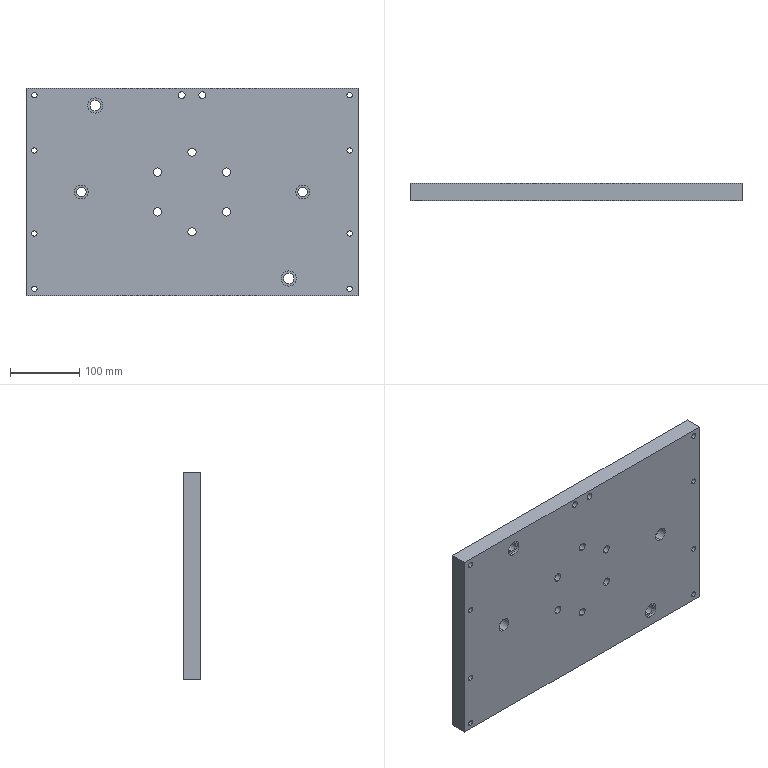Part | STEP file | OP10-020_central plate | 3 solids | 74 faces | box 480 x 25 x 300 mm | volume 3542194 mm3 | cylinder 56 | plane 14 | torus 4 | commonest cylinder face diameters 8 x16 12 x12 22 x8 10 x4 14 x4 15 x4